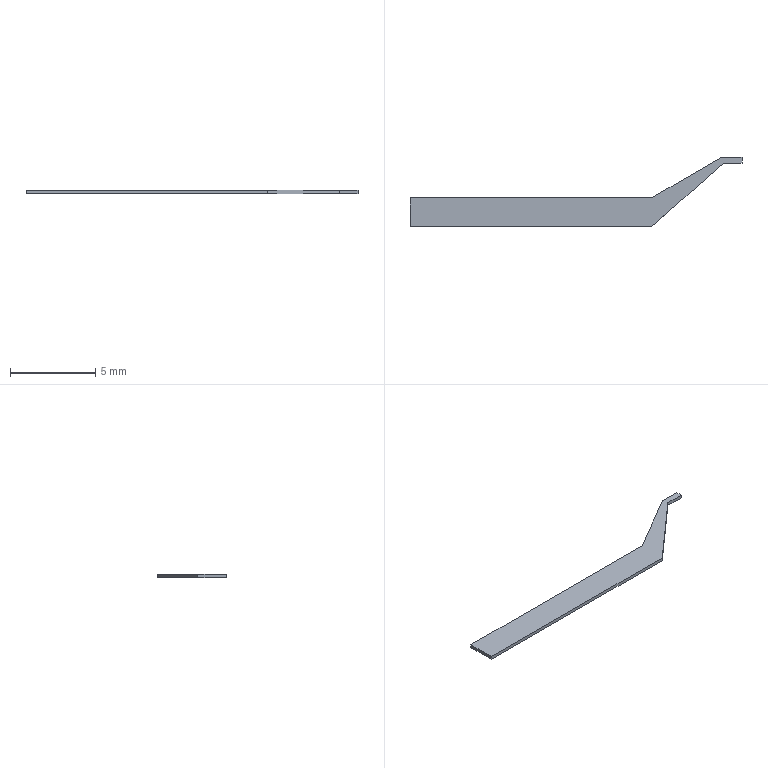Part | SolidWorks | features Extrusion 1 | 1 solid | 10 faces | box 19.5 x 4.08 x 0.2 mm | volume 5.788 mm3 | plane 10
STEP:
#1=CARTESIAN_POINT('',(0.,1.7,0.));
#2=VERTEX_POINT('',#1);
#3=CARTESIAN_POINT('',(0.,0.,0.));
#4=VERTEX_POINT('',#3);
#5=CARTESIAN_POINT('',(0.,0.,0.));
#6=DIRECTION('',(0.,-1.,0.));
#7=VECTOR('',#6,1000.);
#8=LINE('',#5,#7);
#9=EDGE_CURVE('',#2,#4,#8,.T.);
#10=ORIENTED_EDGE('',*,*,#9,.T.);
#11=CARTESIAN_POINT('',(0.,0.,0.2));
#12=VERTEX_POINT('',#11);
#13=CARTESIAN_POINT('',(0.,0.,0.2));
#14=DIRECTION('',(0.,0.,-1.));
#15=VECTOR('',#14,1000.);
#16=LINE('',#13,#15);
#17=EDGE_CURVE('',#12,#4,#16,.T.);
#18=ORIENTED_EDGE('',*,*,#17,.F.);
#19=CARTESIAN_POINT('',(0.,1.7,0.2));
#20=VERTEX_POINT('',#19);
#21=CARTESIAN_POINT('',(0.,0.,0.2));
#22=DIRECTION('',(0.,-1.,0.));
#23=VECTOR('',#22,1000.);
#24=LINE('',#21,#23);
#25=EDGE_CURVE('',#20,#12,#24,.T.);
#26=ORIENTED_EDGE('',*,*,#25,.F.);
#27=CARTESIAN_POINT('',(0.,1.7,0.2));
#28=DIRECTION('',(0.,0.,-1.));
#29=VECTOR('',#28,1000.);
#30=LINE('',#27,#29);
#31=EDGE_CURVE('',#20,#2,#30,.T.);
#32=ORIENTED_EDGE('',*,*,#31,.T.);
#33=EDGE_LOOP('',(#10,#18,#26,#32));
#34=FACE_OUTER_BOUND('',#33,.T.);
#35=CARTESIAN_POINT('',(0.,0.,0.2));
#36=DIRECTION('',(1.,0.,0.));
#37=DIRECTION('',(0.,0.,-1.));
#38=AXIS2_PLACEMENT_3D('',#35,#36,#37);
#39=PLANE('',#38);
#40=ADVANCED_FACE('',(#34),#39,.F.);
#41=CARTESIAN_POINT('',(14.199,0.,0.));
#42=VERTEX_POINT('',#41);
#43=CARTESIAN_POINT('',(0.,0.,0.));
#44=DIRECTION('',(1.,0.,0.));
#45=VECTOR('',#44,1000.);
#46=LINE('',#43,#45);
#47=EDGE_CURVE('',#4,#42,#46,.T.);
#48=ORIENTED_EDGE('',*,*,#47,.T.);
#49=CARTESIAN_POINT('',(14.199,0.,0.2));
#50=VERTEX_POINT('',#49);
#51=CARTESIAN_POINT('',(14.199,0.,0.2));
#52=DIRECTION('',(0.,0.,-1.));
#53=VECTOR('',#52,1000.);
#54=LINE('',#51,#53);
#55=EDGE_CURVE('',#50,#42,#54,.T.);
#56=ORIENTED_EDGE('',*,*,#55,.F.);
#57=CARTESIAN_POINT('',(0.,0.,0.2));
#58=DIRECTION('',(1.,0.,0.));
#59=VECTOR('',#58,1000.);
#60=LINE('',#57,#59);
#61=EDGE_CURVE('',#12,#50,#60,.T.);
#62=ORIENTED_EDGE('',*,*,#61,.F.);
#63=ORIENTED_EDGE('',*,*,#17,.T.);
#64=EDGE_LOOP('',(#48,#56,#62,#63));
#65=FACE_OUTER_BOUND('',#64,.T.);
#66=CARTESIAN_POINT('',(0.,0.,0.2));
#67=DIRECTION('',(0.,1.,0.));
#68=DIRECTION('',(0.,0.,1.));
#69=AXIS2_PLACEMENT_3D('',#66,#67,#68);
#70=PLANE('',#69);
#71=ADVANCED_FACE('',(#65),#70,.F.);
#72=CARTESIAN_POINT('',(18.4,3.73,0.));
#73=VERTEX_POINT('',#72);
#74=CARTESIAN_POINT('',(18.4,3.73,0.));
#75=DIRECTION('',(0.7478,0.6639,0.));
#76=VECTOR('',#75,1000.);
#77=LINE('',#74,#76);
#78=EDGE_CURVE('',#42,#73,#77,.T.);
#79=ORIENTED_EDGE('',*,*,#78,.T.);
#80=CARTESIAN_POINT('',(18.4,3.73,0.2));
#81=VERTEX_POINT('',#80);
#82=CARTESIAN_POINT('',(18.4,3.73,0.2));
#83=DIRECTION('',(0.,0.,-1.));
#84=VECTOR('',#83,1000.);
#85=LINE('',#82,#84);
#86=EDGE_CURVE('',#81,#73,#85,.T.);
#87=ORIENTED_EDGE('',*,*,#86,.F.);
#88=CARTESIAN_POINT('',(18.4,3.73,0.2));
#89=DIRECTION('',(0.7478,0.6639,0.));
#90=VECTOR('',#89,1000.);
#91=LINE('',#88,#90);
#92=EDGE_CURVE('',#50,#81,#91,.T.);
#93=ORIENTED_EDGE('',*,*,#92,.F.);
#94=ORIENTED_EDGE('',*,*,#55,.T.);
#95=EDGE_LOOP('',(#79,#87,#93,#94));
#96=FACE_OUTER_BOUND('',#95,.T.);
#97=CARTESIAN_POINT('',(18.4,3.73,0.2));
#98=DIRECTION('',(-0.6639,0.7478,0.));
#99=DIRECTION('',(-0.7478,-0.6639,0.));
#100=AXIS2_PLACEMENT_3D('',#97,#98,#99);
#101=PLANE('',#100);
#102=ADVANCED_FACE('',(#96),#101,.F.);
#103=CARTESIAN_POINT('',(19.5,3.73,0.));
#104=VERTEX_POINT('',#103);
#105=CARTESIAN_POINT('',(19.5,3.73,0.));
#106=DIRECTION('',(1.,0.,0.));
#107=VECTOR('',#106,1000.);
#108=LINE('',#105,#107);
#109=EDGE_CURVE('',#73,#104,#108,.T.);
#110=ORIENTED_EDGE('',*,*,#109,.T.);
#111=CARTESIAN_POINT('',(19.5,3.73,0.2));
#112=VERTEX_POINT('',#111);
#113=CARTESIAN_POINT('',(19.5,3.73,0.2));
#114=DIRECTION('',(0.,0.,-1.));
#115=VECTOR('',#114,1000.);
#116=LINE('',#113,#115);
#117=EDGE_CURVE('',#112,#104,#116,.T.);
#118=ORIENTED_EDGE('',*,*,#117,.F.);
#119=CARTESIAN_POINT('',(19.5,3.73,0.2));
#120=DIRECTION('',(1.,0.,0.));
#121=VECTOR('',#120,1000.);
#122=LINE('',#119,#121);
#123=EDGE_CURVE('',#81,#112,#122,.T.);
#124=ORIENTED_EDGE('',*,*,#123,.F.);
#125=ORIENTED_EDGE('',*,*,#86,.T.);
#126=EDGE_LOOP('',(#110,#118,#124,#125));
#127=FACE_OUTER_BOUND('',#126,.T.);
#128=CARTESIAN_POINT('',(19.5,3.73,0.2));
#129=DIRECTION('',(0.,1.,0.));
#130=DIRECTION('',(0.,0.,1.));
#131=AXIS2_PLACEMENT_3D('',#128,#129,#130);
#132=PLANE('',#131);
#133=ADVANCED_FACE('',(#127),#132,.F.);
#134=CARTESIAN_POINT('',(19.5,4.08,0.));
#135=VERTEX_POINT('',#134);
#136=CARTESIAN_POINT('',(19.5,3.73,0.));
#137=DIRECTION('',(0.,1.,0.));
#138=VECTOR('',#137,1000.);
#139=LINE('',#136,#138);
#140=EDGE_CURVE('',#104,#135,#139,.T.);
#141=ORIENTED_EDGE('',*,*,#140,.T.);
#142=CARTESIAN_POINT('',(19.5,4.08,0.2));
#143=VERTEX_POINT('',#142);
#144=CARTESIAN_POINT('',(19.5,4.08,0.2));
#145=DIRECTION('',(0.,0.,-1.));
#146=VECTOR('',#145,1000.);
#147=LINE('',#144,#146);
#148=EDGE_CURVE('',#143,#135,#147,.T.);
#149=ORIENTED_EDGE('',*,*,#148,.F.);
#150=CARTESIAN_POINT('',(19.5,3.73,0.2));
#151=DIRECTION('',(0.,1.,0.));
#152=VECTOR('',#151,1000.);
#153=LINE('',#150,#152);
#154=EDGE_CURVE('',#112,#143,#153,.T.);
#155=ORIENTED_EDGE('',*,*,#154,.F.);
#156=ORIENTED_EDGE('',*,*,#117,.T.);
#157=EDGE_LOOP('',(#141,#149,#155,#156));
#158=FACE_OUTER_BOUND('',#157,.T.);
#159=CARTESIAN_POINT('',(19.5,3.73,0.2));
#160=DIRECTION('',(-1.,0.,0.));
#161=DIRECTION('',(0.,0.,1.));
#162=AXIS2_PLACEMENT_3D('',#159,#160,#161);
#163=PLANE('',#162);
#164=ADVANCED_FACE('',(#158),#163,.F.);
#165=CARTESIAN_POINT('',(18.306,4.08,0.));
#166=VERTEX_POINT('',#165);
#167=CARTESIAN_POINT('',(18.306,4.08,0.));
#168=DIRECTION('',(-1.,0.,0.));
#169=VECTOR('',#168,1000.);
#170=LINE('',#167,#169);
#171=EDGE_CURVE('',#135,#166,#170,.T.);
#172=ORIENTED_EDGE('',*,*,#171,.T.);
#173=CARTESIAN_POINT('',(18.306,4.08,0.2));
#174=VERTEX_POINT('',#173);
#175=CARTESIAN_POINT('',(18.306,4.08,0.2));
#176=DIRECTION('',(0.,0.,-1.));
#177=VECTOR('',#176,1000.);
#178=LINE('',#175,#177);
#179=EDGE_CURVE('',#174,#166,#178,.T.);
#180=ORIENTED_EDGE('',*,*,#179,.F.);
#181=CARTESIAN_POINT('',(18.306,4.08,0.2));
#182=DIRECTION('',(-1.,0.,0.));
#183=VECTOR('',#182,1000.);
#184=LINE('',#181,#183);
#185=EDGE_CURVE('',#143,#174,#184,.T.);
#186=ORIENTED_EDGE('',*,*,#185,.F.);
#187=ORIENTED_EDGE('',*,*,#148,.T.);
#188=EDGE_LOOP('',(#172,#180,#186,#187));
#189=FACE_OUTER_BOUND('',#188,.T.);
#190=CARTESIAN_POINT('',(18.306,4.08,0.2));
#191=DIRECTION('',(0.,-1.,0.));
#192=DIRECTION('',(1.,0.,0.));
#193=AXIS2_PLACEMENT_3D('',#190,#191,#192);
#194=PLANE('',#193);
#195=ADVANCED_FACE('',(#189),#194,.F.);
#196=CARTESIAN_POINT('',(14.2,1.7,0.));
#197=VERTEX_POINT('',#196);
#198=CARTESIAN_POINT('',(14.2,1.7,0.));
#199=DIRECTION('',(-0.8652,-0.5015,0.));
#200=VECTOR('',#199,1000.);
#201=LINE('',#198,#200);
#202=EDGE_CURVE('',#166,#197,#201,.T.);
#203=ORIENTED_EDGE('',*,*,#202,.T.);
#204=CARTESIAN_POINT('',(14.2,1.7,0.2));
#205=VERTEX_POINT('',#204);
#206=CARTESIAN_POINT('',(14.2,1.7,0.2));
#207=DIRECTION('',(0.,0.,-1.));
#208=VECTOR('',#207,1000.);
#209=LINE('',#206,#208);
#210=EDGE_CURVE('',#205,#197,#209,.T.);
#211=ORIENTED_EDGE('',*,*,#210,.F.);
#212=CARTESIAN_POINT('',(14.2,1.7,0.2));
#213=DIRECTION('',(-0.8652,-0.5015,0.));
#214=VECTOR('',#213,1000.);
#215=LINE('',#212,#214);
#216=EDGE_CURVE('',#174,#205,#215,.T.);
#217=ORIENTED_EDGE('',*,*,#216,.F.);
#218=ORIENTED_EDGE('',*,*,#179,.T.);
#219=EDGE_LOOP('',(#203,#211,#217,#218));
#220=FACE_OUTER_BOUND('',#219,.T.);
#221=CARTESIAN_POINT('',(14.2,1.7,0.2));
#222=DIRECTION('',(0.5015,-0.8652,0.));
#223=DIRECTION('',(0.8652,0.5015,0.));
#224=AXIS2_PLACEMENT_3D('',#221,#222,#223);
#225=PLANE('',#224);
#226=ADVANCED_FACE('',(#220),#225,.F.);
#227=CARTESIAN_POINT('',(0.,1.7,0.));
#228=DIRECTION('',(-1.,0.,0.));
#229=VECTOR('',#228,1000.);
#230=LINE('',#227,#229);
#231=EDGE_CURVE('',#197,#2,#230,.T.);
#232=ORIENTED_EDGE('',*,*,#231,.T.);
#233=ORIENTED_EDGE('',*,*,#31,.F.);
#234=CARTESIAN_POINT('',(0.,1.7,0.2));
#235=DIRECTION('',(-1.,0.,0.));
#236=VECTOR('',#235,1000.);
#237=LINE('',#234,#236);
#238=EDGE_CURVE('',#205,#20,#237,.T.);
#239=ORIENTED_EDGE('',*,*,#238,.F.);
#240=ORIENTED_EDGE('',*,*,#210,.T.);
#241=EDGE_LOOP('',(#232,#233,#239,#240));
#242=FACE_OUTER_BOUND('',#241,.T.);
#243=CARTESIAN_POINT('',(0.,1.7,0.2));
#244=DIRECTION('',(0.,-1.,0.));
#245=DIRECTION('',(1.,0.,0.));
#246=AXIS2_PLACEMENT_3D('',#243,#244,#245);
#247=PLANE('',#246);
#248=ADVANCED_FACE('',(#242),#247,.F.);
#249=ORIENTED_EDGE('',*,*,#25,.T.);
#250=ORIENTED_EDGE('',*,*,#61,.T.);
#251=ORIENTED_EDGE('',*,*,#92,.T.);
#252=ORIENTED_EDGE('',*,*,#123,.T.);
#253=ORIENTED_EDGE('',*,*,#154,.T.);
#254=ORIENTED_EDGE('',*,*,#185,.T.);
#255=ORIENTED_EDGE('',*,*,#216,.T.);
#256=ORIENTED_EDGE('',*,*,#238,.T.);
#257=EDGE_LOOP('',(#249,#250,#251,#252,#253,#254,#255,#256));
#258=FACE_OUTER_BOUND('',#257,.T.);
#259=CARTESIAN_POINT('',(0.,0.,0.2));
#260=DIRECTION('',(0.,0.,-1.));
#261=DIRECTION('',(-1.,0.,0.));
#262=AXIS2_PLACEMENT_3D('',#259,#260,#261);
#263=PLANE('',#262);
#264=ADVANCED_FACE('',(#258),#263,.F.);
#265=ORIENTED_EDGE('',*,*,#9,.F.);
#266=ORIENTED_EDGE('',*,*,#231,.F.);
#267=ORIENTED_EDGE('',*,*,#202,.F.);
#268=ORIENTED_EDGE('',*,*,#171,.F.);
#269=ORIENTED_EDGE('',*,*,#140,.F.);
#270=ORIENTED_EDGE('',*,*,#109,.F.);
#271=ORIENTED_EDGE('',*,*,#78,.F.);
#272=ORIENTED_EDGE('',*,*,#47,.F.);
#273=EDGE_LOOP('',(#265,#266,#267,#268,#269,#270,#271,#272));
#274=FACE_OUTER_BOUND('',#273,.T.);
#275=CARTESIAN_POINT('',(0.,0.,0.));
#276=DIRECTION('',(0.,0.,-1.));
#277=DIRECTION('',(-1.,0.,0.));
#278=AXIS2_PLACEMENT_3D('',#275,#276,#277);
#279=PLANE('',#278);
#280=ADVANCED_FACE('',(#274),#279,.T.);
#281=CLOSED_SHELL('',(#40,#71,#102,#133,#164,#195,#226,#248,#264,#280));
#282=MANIFOLD_SOLID_BREP('',#281);
#283=CARTESIAN_POINT('',(0.,0.,0.));
#284=DIRECTION('',(0.,0.,1.));
#285=DIRECTION('',(1.,0.,0.));
#286=AXIS2_PLACEMENT_3D('',#283,#284,#285);
#287=(LENGTH_UNIT()NAMED_UNIT(*)SI_UNIT(.MILLI.,.METRE.));
#288=UNCERTAINTY_MEASURE_WITH_UNIT(LENGTH_MEASURE(0.00001),#287,'','');
#289=(NAMED_UNIT(*)PLANE_ANGLE_UNIT()SI_UNIT($,.RADIAN.));
#290=(NAMED_UNIT(*)SI_UNIT($,.STERADIAN.)SOLID_ANGLE_UNIT());
#291=(GEOMETRIC_REPRESENTATION_CONTEXT(3)GLOBAL_UNCERTAINTY_ASSIGNED_CONTEXT((#288))GLOBAL_UNIT_ASSIGNED_CONTEXT((#287,#289,#290))REPRESENTATION_CONTEXT('',''));
#292=ADVANCED_BREP_SHAPE_REPRESENTATION('',(#282,#286),#291);